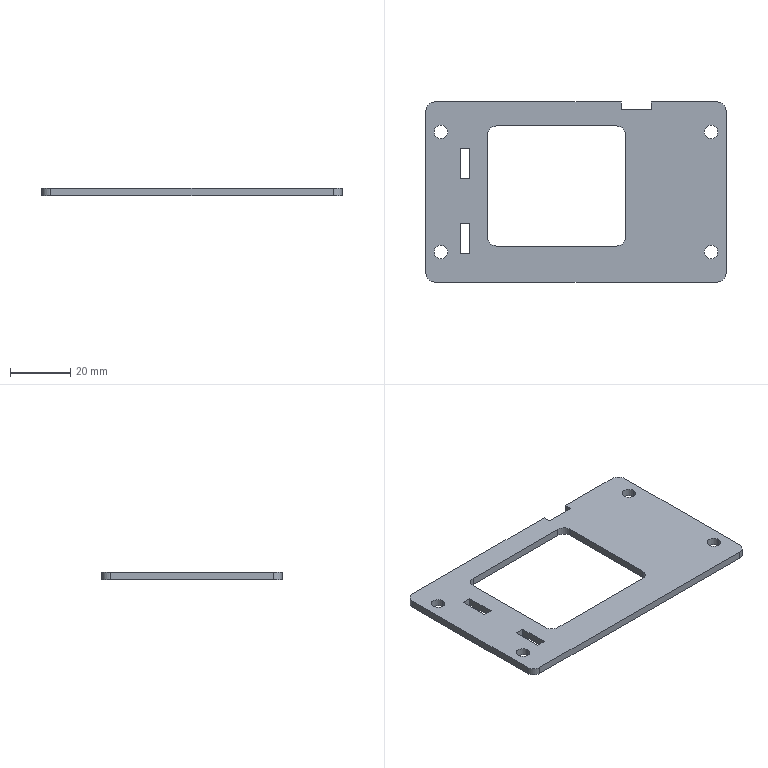Part | SolidWorks | features Cut 2, Fillet 2, ICE 2, MirrorPattern 2, FlatPattern 1, LPattern 1, SMBaseFlange 1, SheetMetal 1 | 1 solid | 38 faces | box 100 x 60 x 2.5 mm | volume 10028 mm3 | plane 22 | cylinder 16 | commonest cylinder face diameters 4.5 x8 6 x8
STEP:
#1=CARTESIAN_POINT('',(-42.75,20.,0.));
#2=VERTEX_POINT('',#1);
#3=CARTESIAN_POINT('',(-47.25,20.,0.));
#4=VERTEX_POINT('',#3);
#5=CARTESIAN_POINT('',(-45.,20.,0.));
#6=DIRECTION('',(0.,0.,-1.));
#7=DIRECTION('',(1.,0.,0.));
#8=AXIS2_PLACEMENT_3D('',#5,#6,#7);
#9=CIRCLE('',#8,2.25);
#10=EDGE_CURVE('',#2,#4,#9,.T.);
#11=ORIENTED_EDGE('',*,*,#10,.F.);
#12=CARTESIAN_POINT('',(-42.75,20.,-2.5));
#13=VERTEX_POINT('',#12);
#14=CARTESIAN_POINT('',(-42.75,20.,7.5));
#15=DIRECTION('',(0.,0.,-1.));
#16=VECTOR('',#15,1000.);
#17=LINE('',#14,#16);
#18=EDGE_CURVE('',#2,#13,#17,.T.);
#19=ORIENTED_EDGE('',*,*,#18,.T.);
#20=CARTESIAN_POINT('',(-47.25,20.,-2.5));
#21=VERTEX_POINT('',#20);
#22=CARTESIAN_POINT('',(-45.,20.,-2.5));
#23=DIRECTION('',(0.,0.,1.));
#24=DIRECTION('',(1.,0.,0.));
#25=AXIS2_PLACEMENT_3D('',#22,#23,#24);
#26=CIRCLE('',#25,2.25);
#27=EDGE_CURVE('',#21,#13,#26,.T.);
#28=ORIENTED_EDGE('',*,*,#27,.F.);
#29=CARTESIAN_POINT('',(-47.25,20.,7.5));
#30=DIRECTION('',(0.,0.,-1.));
#31=VECTOR('',#30,1000.);
#32=LINE('',#29,#31);
#33=EDGE_CURVE('',#4,#21,#32,.T.);
#34=ORIENTED_EDGE('',*,*,#33,.F.);
#35=EDGE_LOOP('',(#11,#19,#28,#34));
#36=FACE_OUTER_BOUND('',#35,.T.);
#37=CARTESIAN_POINT('',(-45.,20.,7.5));
#38=DIRECTION('',(0.,0.,-1.));
#39=DIRECTION('',(-1.,0.,0.));
#40=AXIS2_PLACEMENT_3D('',#37,#38,#39);
#41=CYLINDRICAL_SURFACE('',#40,2.25);
#42=ADVANCED_FACE('',(#36),#41,.F.);
#43=CARTESIAN_POINT('',(-47.25,-20.,0.));
#44=VERTEX_POINT('',#43);
#45=CARTESIAN_POINT('',(-42.75,-20.,0.));
#46=VERTEX_POINT('',#45);
#47=CARTESIAN_POINT('',(-45.,-20.,0.));
#48=DIRECTION('',(0.,0.,1.));
#49=DIRECTION('',(1.,0.,0.));
#50=AXIS2_PLACEMENT_3D('',#47,#48,#49);
#51=CIRCLE('',#50,2.25);
#52=EDGE_CURVE('',#44,#46,#51,.T.);
#53=ORIENTED_EDGE('',*,*,#52,.T.);
#54=CARTESIAN_POINT('',(-42.75,-20.,-2.5));
#55=VERTEX_POINT('',#54);
#56=CARTESIAN_POINT('',(-42.75,-20.,7.5));
#57=DIRECTION('',(0.,0.,-1.));
#58=VECTOR('',#57,1000.);
#59=LINE('',#56,#58);
#60=EDGE_CURVE('',#46,#55,#59,.T.);
#61=ORIENTED_EDGE('',*,*,#60,.T.);
#62=CARTESIAN_POINT('',(-47.25,-20.,-2.5));
#63=VERTEX_POINT('',#62);
#64=CARTESIAN_POINT('',(-45.,-20.,-2.5));
#65=DIRECTION('',(0.,0.,-1.));
#66=DIRECTION('',(1.,0.,0.));
#67=AXIS2_PLACEMENT_3D('',#64,#65,#66);
#68=CIRCLE('',#67,2.25);
#69=EDGE_CURVE('',#55,#63,#68,.T.);
#70=ORIENTED_EDGE('',*,*,#69,.T.);
#71=CARTESIAN_POINT('',(-47.25,-20.,7.5));
#72=DIRECTION('',(0.,0.,-1.));
#73=VECTOR('',#72,1000.);
#74=LINE('',#71,#73);
#75=EDGE_CURVE('',#44,#63,#74,.T.);
#76=ORIENTED_EDGE('',*,*,#75,.F.);
#77=EDGE_LOOP('',(#53,#61,#70,#76));
#78=FACE_OUTER_BOUND('',#77,.T.);
#79=CARTESIAN_POINT('',(-45.,-20.,7.5));
#80=DIRECTION('',(0.,0.,-1.));
#81=DIRECTION('',(-1.,0.,0.));
#82=AXIS2_PLACEMENT_3D('',#79,#80,#81);
#83=CYLINDRICAL_SURFACE('',#82,2.25);
#84=ADVANCED_FACE('',(#78),#83,.F.);
#85=CARTESIAN_POINT('',(47.25,-20.,0.));
#86=VERTEX_POINT('',#85);
#87=CARTESIAN_POINT('',(42.75,-20.,0.));
#88=VERTEX_POINT('',#87);
#89=CARTESIAN_POINT('',(45.,-20.,0.));
#90=DIRECTION('',(0.,0.,-1.));
#91=DIRECTION('',(1.,0.,0.));
#92=AXIS2_PLACEMENT_3D('',#89,#90,#91);
#93=CIRCLE('',#92,2.25);
#94=EDGE_CURVE('',#86,#88,#93,.T.);
#95=ORIENTED_EDGE('',*,*,#94,.F.);
#96=CARTESIAN_POINT('',(47.25,-20.,-2.5));
#97=VERTEX_POINT('',#96);
#98=CARTESIAN_POINT('',(47.25,-20.,7.5));
#99=DIRECTION('',(0.,0.,-1.));
#100=VECTOR('',#99,1000.);
#101=LINE('',#98,#100);
#102=EDGE_CURVE('',#86,#97,#101,.T.);
#103=ORIENTED_EDGE('',*,*,#102,.T.);
#104=CARTESIAN_POINT('',(42.75,-20.,-2.5));
#105=VERTEX_POINT('',#104);
#106=CARTESIAN_POINT('',(45.,-20.,-2.5));
#107=DIRECTION('',(0.,0.,1.));
#108=DIRECTION('',(-1.,0.,0.));
#109=AXIS2_PLACEMENT_3D('',#106,#107,#108);
#110=CIRCLE('',#109,2.25);
#111=EDGE_CURVE('',#105,#97,#110,.T.);
#112=ORIENTED_EDGE('',*,*,#111,.F.);
#113=CARTESIAN_POINT('',(42.75,-20.,7.5));
#114=DIRECTION('',(0.,0.,-1.));
#115=VECTOR('',#114,1000.);
#116=LINE('',#113,#115);
#117=EDGE_CURVE('',#88,#105,#116,.T.);
#118=ORIENTED_EDGE('',*,*,#117,.F.);
#119=EDGE_LOOP('',(#95,#103,#112,#118));
#120=FACE_OUTER_BOUND('',#119,.T.);
#121=CARTESIAN_POINT('',(45.,-20.,7.5));
#122=DIRECTION('',(0.,0.,-1.));
#123=DIRECTION('',(-1.,0.,0.));
#124=AXIS2_PLACEMENT_3D('',#121,#122,#123);
#125=CYLINDRICAL_SURFACE('',#124,2.25);
#126=ADVANCED_FACE('',(#120),#125,.F.);
#127=CARTESIAN_POINT('',(42.75,20.,0.));
#128=VERTEX_POINT('',#127);
#129=CARTESIAN_POINT('',(47.25,20.,0.));
#130=VERTEX_POINT('',#129);
#131=CARTESIAN_POINT('',(45.,20.,0.));
#132=DIRECTION('',(0.,0.,1.));
#133=DIRECTION('',(1.,0.,0.));
#134=AXIS2_PLACEMENT_3D('',#131,#132,#133);
#135=CIRCLE('',#134,2.25);
#136=EDGE_CURVE('',#128,#130,#135,.T.);
#137=ORIENTED_EDGE('',*,*,#136,.T.);
#138=CARTESIAN_POINT('',(47.25,20.,-2.5));
#139=VERTEX_POINT('',#138);
#140=CARTESIAN_POINT('',(47.25,20.,7.5));
#141=DIRECTION('',(0.,0.,-1.));
#142=VECTOR('',#141,1000.);
#143=LINE('',#140,#142);
#144=EDGE_CURVE('',#130,#139,#143,.T.);
#145=ORIENTED_EDGE('',*,*,#144,.T.);
#146=CARTESIAN_POINT('',(42.75,20.,-2.5));
#147=VERTEX_POINT('',#146);
#148=CARTESIAN_POINT('',(45.,20.,-2.5));
#149=DIRECTION('',(0.,0.,-1.));
#150=DIRECTION('',(-1.,0.,0.));
#151=AXIS2_PLACEMENT_3D('',#148,#149,#150);
#152=CIRCLE('',#151,2.25);
#153=EDGE_CURVE('',#139,#147,#152,.T.);
#154=ORIENTED_EDGE('',*,*,#153,.T.);
#155=CARTESIAN_POINT('',(42.75,20.,7.5));
#156=DIRECTION('',(0.,0.,-1.));
#157=VECTOR('',#156,1000.);
#158=LINE('',#155,#157);
#159=EDGE_CURVE('',#128,#147,#158,.T.);
#160=ORIENTED_EDGE('',*,*,#159,.F.);
#161=EDGE_LOOP('',(#137,#145,#154,#160));
#162=FACE_OUTER_BOUND('',#161,.T.);
#163=CARTESIAN_POINT('',(45.,20.,7.5));
#164=DIRECTION('',(0.,0.,-1.));
#165=DIRECTION('',(-1.,0.,0.));
#166=AXIS2_PLACEMENT_3D('',#163,#164,#165);
#167=CYLINDRICAL_SURFACE('',#166,2.25);
#168=ADVANCED_FACE('',(#162),#167,.F.);
#169=CARTESIAN_POINT('',(15.,30.,-2.5));
#170=VERTEX_POINT('',#169);
#171=CARTESIAN_POINT('',(15.,30.,0.));
#172=VERTEX_POINT('',#171);
#173=CARTESIAN_POINT('',(15.,30.,-2.5));
#174=DIRECTION('',(0.,0.,1.));
#175=VECTOR('',#174,1000.);
#176=LINE('',#173,#175);
#177=EDGE_CURVE('',#170,#172,#176,.T.);
#178=ORIENTED_EDGE('',*,*,#177,.F.);
#179=CARTESIAN_POINT('',(-47.,30.,-2.5));
#180=VERTEX_POINT('',#179);
#181=CARTESIAN_POINT('',(-50.,30.,-2.5));
#182=DIRECTION('',(-1.,0.,0.));
#183=VECTOR('',#182,1000.);
#184=LINE('',#181,#183);
#185=EDGE_CURVE('',#170,#180,#184,.T.);
#186=ORIENTED_EDGE('',*,*,#185,.T.);
#187=CARTESIAN_POINT('',(-47.,30.,0.));
#188=VERTEX_POINT('',#187);
#189=CARTESIAN_POINT('',(-47.,30.,-2.5));
#190=DIRECTION('',(0.,0.,1.));
#191=VECTOR('',#190,1000.);
#192=LINE('',#189,#191);
#193=EDGE_CURVE('',#180,#188,#192,.T.);
#194=ORIENTED_EDGE('',*,*,#193,.T.);
#195=CARTESIAN_POINT('',(-50.,30.,0.));
#196=DIRECTION('',(-1.,0.,0.));
#197=VECTOR('',#196,1000.);
#198=LINE('',#195,#197);
#199=EDGE_CURVE('',#172,#188,#198,.T.);
#200=ORIENTED_EDGE('',*,*,#199,.F.);
#201=EDGE_LOOP('',(#178,#186,#194,#200));
#202=FACE_OUTER_BOUND('',#201,.T.);
#203=CARTESIAN_POINT('',(-50.,30.,-2.5));
#204=DIRECTION('',(0.,1.,0.));
#205=DIRECTION('',(0.,0.,1.));
#206=AXIS2_PLACEMENT_3D('',#203,#204,#205);
#207=PLANE('',#206);
#208=ADVANCED_FACE('',(#202),#207,.T.);
#209=CARTESIAN_POINT('',(50.,-27.,0.));
#210=VERTEX_POINT('',#209);
#211=CARTESIAN_POINT('',(50.,27.,0.));
#212=VERTEX_POINT('',#211);
#213=CARTESIAN_POINT('',(50.,30.,0.));
#214=DIRECTION('',(0.,1.,0.));
#215=VECTOR('',#214,1000.);
#216=LINE('',#213,#215);
#217=EDGE_CURVE('',#210,#212,#216,.T.);
#218=ORIENTED_EDGE('',*,*,#217,.F.);
#219=CARTESIAN_POINT('',(50.,-27.,-2.5));
#220=VERTEX_POINT('',#219);
#221=CARTESIAN_POINT('',(50.,-27.,-2.5));
#222=DIRECTION('',(0.,0.,-1.));
#223=VECTOR('',#222,1000.);
#224=LINE('',#221,#223);
#225=EDGE_CURVE('',#210,#220,#224,.T.);
#226=ORIENTED_EDGE('',*,*,#225,.T.);
#227=CARTESIAN_POINT('',(50.,27.,-2.5));
#228=VERTEX_POINT('',#227);
#229=CARTESIAN_POINT('',(50.,30.,-2.5));
#230=DIRECTION('',(0.,1.,0.));
#231=VECTOR('',#230,1000.);
#232=LINE('',#229,#231);
#233=EDGE_CURVE('',#220,#228,#232,.T.);
#234=ORIENTED_EDGE('',*,*,#233,.T.);
#235=CARTESIAN_POINT('',(50.,27.,-2.5));
#236=DIRECTION('',(0.,0.,1.));
#237=VECTOR('',#236,1000.);
#238=LINE('',#235,#237);
#239=EDGE_CURVE('',#228,#212,#238,.T.);
#240=ORIENTED_EDGE('',*,*,#239,.T.);
#241=EDGE_LOOP('',(#218,#226,#234,#240));
#242=FACE_OUTER_BOUND('',#241,.T.);
#243=CARTESIAN_POINT('',(50.,30.,-2.5));
#244=DIRECTION('',(1.,0.,0.));
#245=DIRECTION('',(0.,1.,0.));
#246=AXIS2_PLACEMENT_3D('',#243,#244,#245);
#247=PLANE('',#246);
#248=ADVANCED_FACE('',(#242),#247,.T.);
#249=CARTESIAN_POINT('',(-47.,-30.,0.));
#250=VERTEX_POINT('',#249);
#251=CARTESIAN_POINT('',(47.,-30.,0.));
#252=VERTEX_POINT('',#251);
#253=CARTESIAN_POINT('',(-50.,-30.,0.));
#254=DIRECTION('',(1.,0.,0.));
#255=VECTOR('',#254,1000.);
#256=LINE('',#253,#255);
#257=EDGE_CURVE('',#250,#252,#256,.T.);
#258=ORIENTED_EDGE('',*,*,#257,.F.);
#259=CARTESIAN_POINT('',(-47.,-30.,-2.5));
#260=VERTEX_POINT('',#259);
#261=CARTESIAN_POINT('',(-47.,-30.,-2.5));
#262=DIRECTION('',(0.,0.,-1.));
#263=VECTOR('',#262,1000.);
#264=LINE('',#261,#263);
#265=EDGE_CURVE('',#250,#260,#264,.T.);
#266=ORIENTED_EDGE('',*,*,#265,.T.);
#267=CARTESIAN_POINT('',(47.,-30.,-2.5));
#268=VERTEX_POINT('',#267);
#269=CARTESIAN_POINT('',(-50.,-30.,-2.5));
#270=DIRECTION('',(1.,0.,0.));
#271=VECTOR('',#270,1000.);
#272=LINE('',#269,#271);
#273=EDGE_CURVE('',#260,#268,#272,.T.);
#274=ORIENTED_EDGE('',*,*,#273,.T.);
#275=CARTESIAN_POINT('',(47.,-30.,-2.5));
#276=DIRECTION('',(0.,0.,1.));
#277=VECTOR('',#276,1000.);
#278=LINE('',#275,#277);
#279=EDGE_CURVE('',#268,#252,#278,.T.);
#280=ORIENTED_EDGE('',*,*,#279,.T.);
#281=EDGE_LOOP('',(#258,#266,#274,#280));
#282=FACE_OUTER_BOUND('',#281,.T.);
#283=CARTESIAN_POINT('',(-50.,-30.,-2.5));
#284=DIRECTION('',(0.,-1.,0.));
#285=DIRECTION('',(0.,0.,-1.));
#286=AXIS2_PLACEMENT_3D('',#283,#284,#285);
#287=PLANE('',#286);
#288=ADVANCED_FACE('',(#282),#287,.T.);
#289=CARTESIAN_POINT('',(-50.,27.,-2.5));
#290=VERTEX_POINT('',#289);
#291=CARTESIAN_POINT('',(-50.,-27.,-2.5));
#292=VERTEX_POINT('',#291);
#293=CARTESIAN_POINT('',(-50.,30.,-2.5));
#294=DIRECTION('',(0.,-1.,0.));
#295=VECTOR('',#294,1000.);
#296=LINE('',#293,#295);
#297=EDGE_CURVE('',#290,#292,#296,.T.);
#298=ORIENTED_EDGE('',*,*,#297,.T.);
#299=CARTESIAN_POINT('',(-50.,-27.,0.));
#300=VERTEX_POINT('',#299);
#301=CARTESIAN_POINT('',(-50.,-27.,-2.5));
#302=DIRECTION('',(0.,0.,1.));
#303=VECTOR('',#302,1000.);
#304=LINE('',#301,#303);
#305=EDGE_CURVE('',#292,#300,#304,.T.);
#306=ORIENTED_EDGE('',*,*,#305,.T.);
#307=CARTESIAN_POINT('',(-50.,27.,0.));
#308=VERTEX_POINT('',#307);
#309=CARTESIAN_POINT('',(-50.,30.,0.));
#310=DIRECTION('',(0.,-1.,0.));
#311=VECTOR('',#310,1000.);
#312=LINE('',#309,#311);
#313=EDGE_CURVE('',#308,#300,#312,.T.);
#314=ORIENTED_EDGE('',*,*,#313,.F.);
#315=CARTESIAN_POINT('',(-50.,27.,-2.5));
#316=DIRECTION('',(0.,0.,-1.));
#317=VECTOR('',#316,1000.);
#318=LINE('',#315,#317);
#319=EDGE_CURVE('',#308,#290,#318,.T.);
#320=ORIENTED_EDGE('',*,*,#319,.T.);
#321=EDGE_LOOP('',(#298,#306,#314,#320));
#322=FACE_OUTER_BOUND('',#321,.T.);
#323=CARTESIAN_POINT('',(-50.,30.,-2.5));
#324=DIRECTION('',(-1.,0.,0.));
#325=DIRECTION('',(0.,-1.,0.));
#326=AXIS2_PLACEMENT_3D('',#323,#324,#325);
#327=PLANE('',#326);
#328=ADVANCED_FACE('',(#322),#327,.T.);
#329=CARTESIAN_POINT('',(25.,30.,0.));
#330=VERTEX_POINT('',#329);
#331=CARTESIAN_POINT('',(25.,30.,-2.5));
#332=VERTEX_POINT('',#331);
#333=CARTESIAN_POINT('',(25.,30.,-2.5));
#334=DIRECTION('',(0.,0.,-1.));
#335=VECTOR('',#334,1000.);
#336=LINE('',#333,#335);
#337=EDGE_CURVE('',#330,#332,#336,.T.);
#338=ORIENTED_EDGE('',*,*,#337,.F.);
#339=CARTESIAN_POINT('',(47.,30.,0.));
#340=VERTEX_POINT('',#339);
#341=CARTESIAN_POINT('',(-50.,30.,0.));
#342=DIRECTION('',(-1.,0.,0.));
#343=VECTOR('',#342,1000.);
#344=LINE('',#341,#343);
#345=EDGE_CURVE('',#340,#330,#344,.T.);
#346=ORIENTED_EDGE('',*,*,#345,.F.);
#347=CARTESIAN_POINT('',(47.,30.,-2.5));
#348=VERTEX_POINT('',#347);
#349=CARTESIAN_POINT('',(47.,30.,-2.5));
#350=DIRECTION('',(0.,0.,-1.));
#351=VECTOR('',#350,1000.);
#352=LINE('',#349,#351);
#353=EDGE_CURVE('',#340,#348,#352,.T.);
#354=ORIENTED_EDGE('',*,*,#353,.T.);
#355=CARTESIAN_POINT('',(-50.,30.,-2.5));
#356=DIRECTION('',(-1.,0.,0.));
#357=VECTOR('',#356,1000.);
#358=LINE('',#355,#357);
#359=EDGE_CURVE('',#348,#332,#358,.T.);
#360=ORIENTED_EDGE('',*,*,#359,.T.);
#361=EDGE_LOOP('',(#338,#346,#354,#360));
#362=FACE_OUTER_BOUND('',#361,.T.);
#363=CARTESIAN_POINT('',(-50.,30.,-2.5));
#364=DIRECTION('',(0.,1.,0.));
#365=DIRECTION('',(0.,0.,1.));
#366=AXIS2_PLACEMENT_3D('',#363,#364,#365);
#367=PLANE('',#366);
#368=ADVANCED_FACE('',(#362),#367,.T.);
#369=CARTESIAN_POINT('',(-26.5,22.,-2.5));
#370=VERTEX_POINT('',#369);
#371=CARTESIAN_POINT('',(13.5,22.,-2.5));
#372=VERTEX_POINT('',#371);
#373=CARTESIAN_POINT('',(-29.5,22.,-2.5));
#374=DIRECTION('',(1.,0.,0.));
#375=VECTOR('',#374,1000.);
#376=LINE('',#373,#375);
#377=EDGE_CURVE('',#370,#372,#376,.T.);
#378=ORIENTED_EDGE('',*,*,#377,.F.);
#379=CARTESIAN_POINT('',(-29.5,19.,-2.5));
#380=VERTEX_POINT('',#379);
#381=CARTESIAN_POINT('',(-26.5,19.,-2.5));
#382=DIRECTION('',(0.,0.,1.));
#383=DIRECTION('',(1.,0.,0.));
#384=AXIS2_PLACEMENT_3D('',#381,#382,#383);
#385=CIRCLE('',#384,3.);
#386=EDGE_CURVE('',#370,#380,#385,.T.);
#387=ORIENTED_EDGE('',*,*,#386,.T.);
#388=CARTESIAN_POINT('',(-29.5,-15.,-2.5));
#389=VERTEX_POINT('',#388);
#390=CARTESIAN_POINT('',(-29.5,-18.,-2.5));
#391=DIRECTION('',(0.,1.,0.));
#392=VECTOR('',#391,1000.);
#393=LINE('',#390,#392);
#394=EDGE_CURVE('',#389,#380,#393,.T.);
#395=ORIENTED_EDGE('',*,*,#394,.F.);
#396=CARTESIAN_POINT('',(-26.5,-18.,-2.5));
#397=VERTEX_POINT('',#396);
#398=CARTESIAN_POINT('',(-26.5,-15.,-2.5));
#399=DIRECTION('',(0.,0.,1.));
#400=DIRECTION('',(1.,0.,0.));
#401=AXIS2_PLACEMENT_3D('',#398,#399,#400);
#402=CIRCLE('',#401,3.);
#403=EDGE_CURVE('',#389,#397,#402,.T.);
#404=ORIENTED_EDGE('',*,*,#403,.T.);
#405=CARTESIAN_POINT('',(13.5,-18.,-2.5));
#406=VERTEX_POINT('',#405);
#407=CARTESIAN_POINT('',(-29.5,-18.,-2.5));
#408=DIRECTION('',(-1.,0.,0.));
#409=VECTOR('',#408,1000.);
#410=LINE('',#407,#409);
#411=EDGE_CURVE('',#406,#397,#410,.T.);
#412=ORIENTED_EDGE('',*,*,#411,.F.);
#413=CARTESIAN_POINT('',(16.5,-15.,-2.5));
#414=VERTEX_POINT('',#413);
#415=CARTESIAN_POINT('',(13.5,-15.,-2.5));
#416=DIRECTION('',(0.,0.,1.));
#417=DIRECTION('',(1.,0.,0.));
#418=AXIS2_PLACEMENT_3D('',#415,#416,#417);
#419=CIRCLE('',#418,3.);
#420=EDGE_CURVE('',#406,#414,#419,.T.);
#421=ORIENTED_EDGE('',*,*,#420,.T.);
#422=CARTESIAN_POINT('',(16.5,19.,-2.5));
#423=VERTEX_POINT('',#422);
#424=CARTESIAN_POINT('',(16.5,-18.,-2.5));
#425=DIRECTION('',(0.,-1.,0.));
#426=VECTOR('',#425,1000.);
#427=LINE('',#424,#426);
#428=EDGE_CURVE('',#423,#414,#427,.T.);
#429=ORIENTED_EDGE('',*,*,#428,.F.);
#430=CARTESIAN_POINT('',(13.5,19.,-2.5));
#431=DIRECTION('',(0.,0.,1.));
#432=DIRECTION('',(1.,0.,0.));
#433=AXIS2_PLACEMENT_3D('',#430,#431,#432);
#434=CIRCLE('',#433,3.);
#435=EDGE_CURVE('',#423,#372,#434,.T.);
#436=ORIENTED_EDGE('',*,*,#435,.T.);
#437=EDGE_LOOP('',(#378,#387,#395,#404,#412,#421,#429,#436));
#438=FACE_BOUND('',#437,.T.);
#439=ORIENTED_EDGE('',*,*,#27,.T.);
#440=CARTESIAN_POINT('',(-45.,20.,-2.5));
#441=DIRECTION('',(0.,0.,1.));
#442=DIRECTION('',(1.,0.,0.));
#443=AXIS2_PLACEMENT_3D('',#440,#441,#442);
#444=CIRCLE('',#443,2.25);
#445=EDGE_CURVE('',#13,#21,#444,.T.);
#446=ORIENTED_EDGE('',*,*,#445,.T.);
#447=EDGE_LOOP('',(#439,#446));
#448=FACE_BOUND('',#447,.T.);
#449=CARTESIAN_POINT('',(-45.,-20.,-2.5));
#450=DIRECTION('',(0.,0.,-1.));
#451=DIRECTION('',(1.,0.,0.));
#452=AXIS2_PLACEMENT_3D('',#449,#450,#451);
#453=CIRCLE('',#452,2.25);
#454=EDGE_CURVE('',#63,#55,#453,.T.);
#455=ORIENTED_EDGE('',*,*,#454,.F.);
#456=ORIENTED_EDGE('',*,*,#69,.F.);
#457=EDGE_LOOP('',(#455,#456));
#458=FACE_BOUND('',#457,.T.);
#459=ORIENTED_EDGE('',*,*,#111,.T.);
#460=CARTESIAN_POINT('',(45.,-20.,-2.5));
#461=DIRECTION('',(0.,0.,1.));
#462=DIRECTION('',(-1.,0.,0.));
#463=AXIS2_PLACEMENT_3D('',#460,#461,#462);
#464=CIRCLE('',#463,2.25);
#465=EDGE_CURVE('',#97,#105,#464,.T.);
#466=ORIENTED_EDGE('',*,*,#465,.T.);
#467=EDGE_LOOP('',(#459,#466));
#468=FACE_BOUND('',#467,.T.);
#469=CARTESIAN_POINT('',(45.,20.,-2.5));
#470=DIRECTION('',(0.,0.,-1.));
#471=DIRECTION('',(-1.,0.,0.));
#472=AXIS2_PLACEMENT_3D('',#469,#470,#471);
#473=CIRCLE('',#472,2.25);
#474=EDGE_CURVE('',#147,#139,#473,.T.);
#475=ORIENTED_EDGE('',*,*,#474,.F.);
#476=ORIENTED_EDGE('',*,*,#153,.F.);
#477=EDGE_LOOP('',(#475,#476));
#478=FACE_BOUND('',#477,.T.);
#479=CARTESIAN_POINT('',(-35.5,-20.5,-2.5));
#480=VERTEX_POINT('',#479);
#481=CARTESIAN_POINT('',(-38.5,-20.5,-2.5));
#482=VERTEX_POINT('',#481);
#483=CARTESIAN_POINT('',(-35.5,-20.5,-2.5));
#484=DIRECTION('',(-1.,0.,0.));
#485=VECTOR('',#484,1000.);
#486=LINE('',#483,#485);
#487=EDGE_CURVE('',#480,#482,#486,.T.);
#488=ORIENTED_EDGE('',*,*,#487,.F.);
#489=CARTESIAN_POINT('',(-35.5,-10.5,-2.5));
#490=VERTEX_POINT('',#489);
#491=CARTESIAN_POINT('',(-35.5,-20.5,-2.5));
#492=DIRECTION('',(0.,-1.,0.));
#493=VECTOR('',#492,1000.);
#494=LINE('',#491,#493);
#495=EDGE_CURVE('',#490,#480,#494,.T.);
#496=ORIENTED_EDGE('',*,*,#495,.F.);
#497=CARTESIAN_POINT('',(-38.5,-10.5,-2.5));
#498=VERTEX_POINT('',#497);
#499=CARTESIAN_POINT('',(-35.5,-10.5,-2.5));
#500=DIRECTION('',(1.,0.,0.));
#501=VECTOR('',#500,1000.);
#502=LINE('',#499,#501);
#503=EDGE_CURVE('',#498,#490,#502,.T.);
#504=ORIENTED_EDGE('',*,*,#503,.F.);
#505=CARTESIAN_POINT('',(-38.5,-20.5,-2.5));
#506=DIRECTION('',(0.,1.,0.));
#507=VECTOR('',#506,1000.);
#508=LINE('',#505,#507);
#509=EDGE_CURVE('',#482,#498,#508,.T.);
#510=ORIENTED_EDGE('',*,*,#509,.F.);
#511=EDGE_LOOP('',(#488,#496,#504,#510));
#512=FACE_BOUND('',#511,.T.);
#513=CARTESIAN_POINT('',(-35.5,4.5,-2.5));
#514=VERTEX_POINT('',#513);
#515=CARTESIAN_POINT('',(-38.5,4.5,-2.5));
#516=VERTEX_POINT('',#515);
#517=CARTESIAN_POINT('',(-35.5,4.5,-2.5));
#518=DIRECTION('',(-1.,0.,0.));
#519=VECTOR('',#518,1000.);
#520=LINE('',#517,#519);
#521=EDGE_CURVE('',#514,#516,#520,.T.);
#522=ORIENTED_EDGE('',*,*,#521,.F.);
#523=CARTESIAN_POINT('',(-35.5,14.5,-2.5));
#524=VERTEX_POINT('',#523);
#525=CARTESIAN_POINT('',(-35.5,4.5,-2.5));
#526=DIRECTION('',(0.,-1.,0.));
#527=VECTOR('',#526,1000.);
#528=LINE('',#525,#527);
#529=EDGE_CURVE('',#524,#514,#528,.T.);
#530=ORIENTED_EDGE('',*,*,#529,.F.);
#531=CARTESIAN_POINT('',(-38.5,14.5,-2.5));
#532=VERTEX_POINT('',#531);
#533=CARTESIAN_POINT('',(-35.5,14.5,-2.5));
#534=DIRECTION('',(1.,0.,0.));
#535=VECTOR('',#534,1000.);
#536=LINE('',#533,#535);
#537=EDGE_CURVE('',#532,#524,#536,.T.);
#538=ORIENTED_EDGE('',*,*,#537,.F.);
#539=CARTESIAN_POINT('',(-38.5,4.5,-2.5));
#540=DIRECTION('',(0.,1.,0.));
#541=VECTOR('',#540,1000.);
#542=LINE('',#539,#541);
#543=EDGE_CURVE('',#516,#532,#542,.T.);
#544=ORIENTED_EDGE('',*,*,#543,.F.);
#545=EDGE_LOOP('',(#522,#530,#538,#544));
#546=FACE_BOUND('',#545,.T.);
#547=ORIENTED_EDGE('',*,*,#185,.F.);
#548=CARTESIAN_POINT('',(15.,27.5,-2.5));
#549=VERTEX_POINT('',#548);
#550=CARTESIAN_POINT('',(15.,0.,-2.5));
#551=DIRECTION('',(0.,-1.,0.));
#552=VECTOR('',#551,1000.);
#553=LINE('',#550,#552);
#554=EDGE_CURVE('',#170,#549,#553,.T.);
#555=ORIENTED_EDGE('',*,*,#554,.T.);
#556=CARTESIAN_POINT('',(25.,27.5,-2.5));
#557=VERTEX_POINT('',#556);
#558=CARTESIAN_POINT('',(0.,27.5,-2.5));
#559=DIRECTION('',(1.,0.,0.));
#560=VECTOR('',#559,1000.);
#561=LINE('',#558,#560);
#562=EDGE_CURVE('',#549,#557,#561,.T.);
#563=ORIENTED_EDGE('',*,*,#562,.T.);
#564=CARTESIAN_POINT('',(25.,0.,-2.5));
#565=DIRECTION('',(0.,1.,0.));
#566=VECTOR('',#565,1000.);
#567=LINE('',#564,#566);
#568=EDGE_CURVE('',#557,#332,#567,.T.);
#569=ORIENTED_EDGE('',*,*,#568,.T.);
#570=ORIENTED_EDGE('',*,*,#359,.F.);
#571=CARTESIAN_POINT('',(47.,27.,-2.5));
#572=DIRECTION('',(0.,0.,-1.));
#573=DIRECTION('',(1.,0.,0.));
#574=AXIS2_PLACEMENT_3D('',#571,#572,#573);
#575=CIRCLE('',#574,3.);
#576=EDGE_CURVE('',#348,#228,#575,.T.);
#577=ORIENTED_EDGE('',*,*,#576,.T.);
#578=ORIENTED_EDGE('',*,*,#233,.F.);
#579=CARTESIAN_POINT('',(47.,-27.,-2.5));
#580=DIRECTION('',(0.,0.,-1.));
#581=DIRECTION('',(1.,0.,0.));
#582=AXIS2_PLACEMENT_3D('',#579,#580,#581);
#583=CIRCLE('',#582,3.);
#584=EDGE_CURVE('',#220,#268,#583,.T.);
#585=ORIENTED_EDGE('',*,*,#584,.T.);
#586=ORIENTED_EDGE('',*,*,#273,.F.);
#587=CARTESIAN_POINT('',(-47.,-27.,-2.5));
#588=DIRECTION('',(0.,0.,-1.));
#589=DIRECTION('',(1.,0.,0.));
#590=AXIS2_PLACEMENT_3D('',#587,#588,#589);
#591=CIRCLE('',#590,3.);
#592=EDGE_CURVE('',#260,#292,#591,.T.);
#593=ORIENTED_EDGE('',*,*,#592,.T.);
#594=ORIENTED_EDGE('',*,*,#297,.F.);
#595=CARTESIAN_POINT('',(-47.,27.,-2.5));
#596=DIRECTION('',(0.,0.,-1.));
#597=DIRECTION('',(1.,0.,0.));
#598=AXIS2_PLACEMENT_3D('',#595,#596,#597);
#599=CIRCLE('',#598,3.);
#600=EDGE_CURVE('',#290,#180,#599,.T.);
#601=ORIENTED_EDGE('',*,*,#600,.T.);
#602=EDGE_LOOP('',(#547,#555,#563,#569,#570,#577,#578,#585,#586,#593,#594,#601));
#603=FACE_OUTER_BOUND('',#602,.T.);
#604=CARTESIAN_POINT('',(0.,0.,-2.5));
#605=DIRECTION('',(0.,0.,1.));
#606=DIRECTION('',(1.,0.,0.));
#607=AXIS2_PLACEMENT_3D('',#604,#605,#606);
#608=PLANE('',#607);
#609=ADVANCED_FACE('',(#438,#448,#458,#468,#478,#512,#546,#603),#608,.F.);
#610=CARTESIAN_POINT('',(-29.5,19.,0.));
#611=VERTEX_POINT('',#610);
#612=CARTESIAN_POINT('',(-29.5,-15.,0.));
#613=VERTEX_POINT('',#612);
#614=CARTESIAN_POINT('',(-29.5,0.,0.));
#615=DIRECTION('',(0.,-1.,0.));
#616=VECTOR('',#615,1000.);
#617=LINE('',#614,#616);
#618=EDGE_CURVE('',#611,#613,#617,.T.);
#619=ORIENTED_EDGE('',*,*,#618,.F.);
#620=CARTESIAN_POINT('',(-26.5,22.,0.));
#621=VERTEX_POINT('',#620);
#622=CARTESIAN_POINT('',(-26.5,19.,0.));
#623=DIRECTION('',(0.,0.,-1.));
#624=DIRECTION('',(1.,0.,0.));
#625=AXIS2_PLACEMENT_3D('',#622,#623,#624);
#626=CIRCLE('',#625,3.);
#627=EDGE_CURVE('',#611,#621,#626,.T.);
#628=ORIENTED_EDGE('',*,*,#627,.T.);
#629=CARTESIAN_POINT('',(13.5,22.,0.));
#630=VERTEX_POINT('',#629);
#631=CARTESIAN_POINT('',(0.,22.,0.));
#632=DIRECTION('',(-1.,0.,0.));
#633=VECTOR('',#632,1000.);
#634=LINE('',#631,#633);
#635=EDGE_CURVE('',#630,#621,#634,.T.);
#636=ORIENTED_EDGE('',*,*,#635,.F.);
#637=CARTESIAN_POINT('',(16.5,19.,0.));
#638=VERTEX_POINT('',#637);
#639=CARTESIAN_POINT('',(13.5,19.,0.));
#640=DIRECTION('',(0.,0.,-1.));
#641=DIRECTION('',(1.,0.,0.));
#642=AXIS2_PLACEMENT_3D('',#639,#640,#641);
#643=CIRCLE('',#642,3.);
#644=EDGE_CURVE('',#630,#638,#643,.T.);
#645=ORIENTED_EDGE('',*,*,#644,.T.);
#646=CARTESIAN_POINT('',(16.5,-15.,0.));
#647=VERTEX_POINT('',#646);
#648=CARTESIAN_POINT('',(16.5,0.,0.));
#649=DIRECTION('',(0.,1.,0.));
#650=VECTOR('',#649,1000.);
#651=LINE('',#648,#650);
#652=EDGE_CURVE('',#647,#638,#651,.T.);
#653=ORIENTED_EDGE('',*,*,#652,.F.);
#654=CARTESIAN_POINT('',(13.5,-18.,0.));
#655=VERTEX_POINT('',#654);
#656=CARTESIAN_POINT('',(13.5,-15.,0.));
#657=DIRECTION('',(0.,0.,-1.));
#658=DIRECTION('',(1.,0.,0.));
#659=AXIS2_PLACEMENT_3D('',#656,#657,#658);
#660=CIRCLE('',#659,3.);
#661=EDGE_CURVE('',#647,#655,#660,.T.);
#662=ORIENTED_EDGE('',*,*,#661,.T.);
#663=CARTESIAN_POINT('',(-26.5,-18.,0.));
#664=VERTEX_POINT('',#663);
#665=CARTESIAN_POINT('',(0.,-18.,0.));
#666=DIRECTION('',(1.,0.,0.));
#667=VECTOR('',#666,1000.);
#668=LINE('',#665,#667);
#669=EDGE_CURVE('',#664,#655,#668,.T.);
#670=ORIENTED_EDGE('',*,*,#669,.F.);
#671=CARTESIAN_POINT('',(-26.5,-15.,0.));
#672=DIRECTION('',(0.,0.,-1.));
#673=DIRECTION('',(1.,0.,0.));
#674=AXIS2_PLACEMENT_3D('',#671,#672,#673);
#675=CIRCLE('',#674,3.);
#676=EDGE_CURVE('',#664,#613,#675,.T.);
#677=ORIENTED_EDGE('',*,*,#676,.T.);
#678=EDGE_LOOP('',(#619,#628,#636,#645,#653,#662,#670,#677));
#679=FACE_BOUND('',#678,.T.);
#680=CARTESIAN_POINT('',(-45.,20.,0.));
#681=DIRECTION('',(0.,0.,-1.));
#682=DIRECTION('',(1.,0.,0.));
#683=AXIS2_PLACEMENT_3D('',#680,#681,#682);
#684=CIRCLE('',#683,2.25);
#685=EDGE_CURVE('',#4,#2,#684,.T.);
#686=ORIENTED_EDGE('',*,*,#685,.T.);
#687=ORIENTED_EDGE('',*,*,#10,.T.);
#688=EDGE_LOOP('',(#686,#687));
#689=FACE_BOUND('',#688,.T.);
#690=ORIENTED_EDGE('',*,*,#52,.F.);
#691=CARTESIAN_POINT('',(-45.,-20.,0.));
#692=DIRECTION('',(0.,0.,1.));
#693=DIRECTION('',(1.,0.,0.));
#694=AXIS2_PLACEMENT_3D('',#691,#692,#693);
#695=CIRCLE('',#694,2.25);
#696=EDGE_CURVE('',#46,#44,#695,.T.);
#697=ORIENTED_EDGE('',*,*,#696,.F.);
#698=EDGE_LOOP('',(#690,#697));
#699=FACE_BOUND('',#698,.T.);
#700=CARTESIAN_POINT('',(45.,-20.,0.));
#701=DIRECTION('',(0.,0.,-1.));
#702=DIRECTION('',(1.,0.,0.));
#703=AXIS2_PLACEMENT_3D('',#700,#701,#702);
#704=CIRCLE('',#703,2.25);
#705=EDGE_CURVE('',#88,#86,#704,.T.);
#706=ORIENTED_EDGE('',*,*,#705,.T.);
#707=ORIENTED_EDGE('',*,*,#94,.T.);
#708=EDGE_LOOP('',(#706,#707));
#709=FACE_BOUND('',#708,.T.);
#710=ORIENTED_EDGE('',*,*,#136,.F.);
#711=CARTESIAN_POINT('',(45.,20.,0.));
#712=DIRECTION('',(0.,0.,1.));
#713=DIRECTION('',(1.,0.,0.));
#714=AXIS2_PLACEMENT_3D('',#711,#712,#713);
#715=CIRCLE('',#714,2.25);
#716=EDGE_CURVE('',#130,#128,#715,.T.);
#717=ORIENTED_EDGE('',*,*,#716,.F.);
#718=EDGE_LOOP('',(#710,#717));
#719=FACE_BOUND('',#718,.T.);
#720=CARTESIAN_POINT('',(-35.5,-20.5,0.));
#721=VERTEX_POINT('',#720);
#722=CARTESIAN_POINT('',(-35.5,-10.5,0.));
#723=VERTEX_POINT('',#722);
#724=CARTESIAN_POINT('',(-35.5,0.,0.));
#725=DIRECTION('',(0.,1.,0.));
#726=VECTOR('',#725,1000.);
#727=LINE('',#724,#726);
#728=EDGE_CURVE('',#721,#723,#727,.T.);
#729=ORIENTED_EDGE('',*,*,#728,.F.);
#730=CARTESIAN_POINT('',(-38.5,-20.5,0.));
#731=VERTEX_POINT('',#730);
#732=CARTESIAN_POINT('',(0.,-20.5,0.));
#733=DIRECTION('',(1.,0.,0.));
#734=VECTOR('',#733,1000.);
#735=LINE('',#732,#734);
#736=EDGE_CURVE('',#731,#721,#735,.T.);
#737=ORIENTED_EDGE('',*,*,#736,.F.);
#738=CARTESIAN_POINT('',(-38.5,-10.5,0.));
#739=VERTEX_POINT('',#738);
#740=CARTESIAN_POINT('',(-38.5,0.,0.));
#741=DIRECTION('',(0.,-1.,0.));
#742=VECTOR('',#741,1000.);
#743=LINE('',#740,#742);
#744=EDGE_CURVE('',#739,#731,#743,.T.);
#745=ORIENTED_EDGE('',*,*,#744,.F.);
#746=CARTESIAN_POINT('',(0.,-10.5,0.));
#747=DIRECTION('',(-1.,0.,0.));
#748=VECTOR('',#747,1000.);
#749=LINE('',#746,#748);
#750=EDGE_CURVE('',#723,#739,#749,.T.);
#751=ORIENTED_EDGE('',*,*,#750,.F.);
#752=EDGE_LOOP('',(#729,#737,#745,#751));
#753=FACE_BOUND('',#752,.T.);
#754=CARTESIAN_POINT('',(-35.5,4.5,0.));
#755=VERTEX_POINT('',#754);
#756=CARTESIAN_POINT('',(-35.5,14.5,0.));
#757=VERTEX_POINT('',#756);
#758=CARTESIAN_POINT('',(-35.5,0.,0.));
#759=DIRECTION('',(0.,1.,0.));
#760=VECTOR('',#759,1000.);
#761=LINE('',#758,#760);
#762=EDGE_CURVE('',#755,#757,#761,.T.);
#763=ORIENTED_EDGE('',*,*,#762,.F.);
#764=CARTESIAN_POINT('',(-38.5,4.5,0.));
#765=VERTEX_POINT('',#764);
#766=CARTESIAN_POINT('',(0.,4.5,0.));
#767=DIRECTION('',(1.,0.,0.));
#768=VECTOR('',#767,1000.);
#769=LINE('',#766,#768);
#770=EDGE_CURVE('',#765,#755,#769,.T.);
#771=ORIENTED_EDGE('',*,*,#770,.F.);
#772=CARTESIAN_POINT('',(-38.5,14.5,0.));
#773=VERTEX_POINT('',#772);
#774=CARTESIAN_POINT('',(-38.5,0.,0.));
#775=DIRECTION('',(0.,-1.,0.));
#776=VECTOR('',#775,1000.);
#777=LINE('',#774,#776);
#778=EDGE_CURVE('',#773,#765,#777,.T.);
#779=ORIENTED_EDGE('',*,*,#778,.F.);
#780=CARTESIAN_POINT('',(0.,14.5,0.));
#781=DIRECTION('',(-1.,0.,0.));
#782=VECTOR('',#781,1000.);
#783=LINE('',#780,#782);
#784=EDGE_CURVE('',#757,#773,#783,.T.);
#785=ORIENTED_EDGE('',*,*,#784,.F.);
#786=EDGE_LOOP('',(#763,#771,#779,#785));
#787=FACE_BOUND('',#786,.T.);
#788=CARTESIAN_POINT('',(15.,27.5,0.));
#789=VERTEX_POINT('',#788);
#790=CARTESIAN_POINT('',(15.,0.,0.));
#791=DIRECTION('',(0.,-1.,0.));
#792=VECTOR('',#791,1000.);
#793=LINE('',#790,#792);
#794=EDGE_CURVE('',#172,#789,#793,.T.);
#795=ORIENTED_EDGE('',*,*,#794,.F.);
#796=ORIENTED_EDGE('',*,*,#199,.T.);
#797=CARTESIAN_POINT('',(-47.,27.,0.));
#798=DIRECTION('',(0.,0.,1.));
#799=DIRECTION('',(1.,0.,0.));
#800=AXIS2_PLACEMENT_3D('',#797,#798,#799);
#801=CIRCLE('',#800,3.);
#802=EDGE_CURVE('',#188,#308,#801,.T.);
#803=ORIENTED_EDGE('',*,*,#802,.T.);
#804=ORIENTED_EDGE('',*,*,#313,.T.);
#805=CARTESIAN_POINT('',(-47.,-27.,0.));
#806=DIRECTION('',(0.,0.,1.));
#807=DIRECTION('',(1.,0.,0.));
#808=AXIS2_PLACEMENT_3D('',#805,#806,#807);
#809=CIRCLE('',#808,3.);
#810=EDGE_CURVE('',#300,#250,#809,.T.);
#811=ORIENTED_EDGE('',*,*,#810,.T.);
#812=ORIENTED_EDGE('',*,*,#257,.T.);
#813=CARTESIAN_POINT('',(47.,-27.,0.));
#814=DIRECTION('',(0.,0.,1.));
#815=DIRECTION('',(1.,0.,0.));
#816=AXIS2_PLACEMENT_3D('',#813,#814,#815);
#817=CIRCLE('',#816,3.);
#818=EDGE_CURVE('',#252,#210,#817,.T.);
#819=ORIENTED_EDGE('',*,*,#818,.T.);
#820=ORIENTED_EDGE('',*,*,#217,.T.);
#821=CARTESIAN_POINT('',(47.,27.,0.));
#822=DIRECTION('',(0.,0.,1.));
#823=DIRECTION('',(1.,0.,0.));
#824=AXIS2_PLACEMENT_3D('',#821,#822,#823);
#825=CIRCLE('',#824,3.);
#826=EDGE_CURVE('',#212,#340,#825,.T.);
#827=ORIENTED_EDGE('',*,*,#826,.T.);
#828=ORIENTED_EDGE('',*,*,#345,.T.);
#829=CARTESIAN_POINT('',(25.,27.5,0.));
#830=VERTEX_POINT('',#829);
#831=CARTESIAN_POINT('',(25.,33.638,0.));
#832=DIRECTION('',(0.,1.,0.));
#833=VECTOR('',#832,1000.);
#834=LINE('',#831,#833);
#835=EDGE_CURVE('',#830,#330,#834,.T.);
#836=ORIENTED_EDGE('',*,*,#835,.F.);
#837=CARTESIAN_POINT('',(15.,27.5,0.));
#838=DIRECTION('',(1.,0.,0.));
#839=VECTOR('',#838,1000.);
#840=LINE('',#837,#839);
#841=EDGE_CURVE('',#789,#830,#840,.T.);
#842=ORIENTED_EDGE('',*,*,#841,.F.);
#843=EDGE_LOOP('',(#795,#796,#803,#804,#811,#812,#819,#820,#827,#828,#836,#842));
#844=FACE_OUTER_BOUND('',#843,.T.);
#845=CARTESIAN_POINT('',(0.,0.,0.));
#846=DIRECTION('',(0.,0.,1.));
#847=DIRECTION('',(1.,0.,0.));
#848=AXIS2_PLACEMENT_3D('',#845,#846,#847);
#849=PLANE('',#848);
#850=ADVANCED_FACE('',(#679,#689,#699,#709,#719,#753,#787,#844),#849,.T.);
#851=ORIENTED_EDGE('',*,*,#592,.F.);
#852=ORIENTED_EDGE('',*,*,#265,.F.);
#853=ORIENTED_EDGE('',*,*,#810,.F.);
#854=ORIENTED_EDGE('',*,*,#305,.F.);
#855=EDGE_LOOP('',(#851,#852,#853,#854));
#856=FACE_OUTER_BOUND('',#855,.T.);
#857=CARTESIAN_POINT('',(-47.,-27.,-2.5));
#858=DIRECTION('',(0.,0.,1.));
#859=DIRECTION('',(1.,0.,0.));
#860=AXIS2_PLACEMENT_3D('',#857,#858,#859);
#861=CYLINDRICAL_SURFACE('',#860,3.);
#862=ADVANCED_FACE('',(#856),#861,.T.);
#863=ORIENTED_EDGE('',*,*,#584,.F.);
#864=ORIENTED_EDGE('',*,*,#225,.F.);
#865=ORIENTED_EDGE('',*,*,#818,.F.);
#866=ORIENTED_EDGE('',*,*,#279,.F.);
#867=EDGE_LOOP('',(#863,#864,#865,#866));
#868=FACE_OUTER_BOUND('',#867,.T.);
#869=CARTESIAN_POINT('',(47.,-27.,-2.5));
#870=DIRECTION('',(0.,0.,1.));
#871=DIRECTION('',(1.,0.,0.));
#872=AXIS2_PLACEMENT_3D('',#869,#870,#871);
#873=CYLINDRICAL_SURFACE('',#872,3.);
#874=ADVANCED_FACE('',(#868),#873,.T.);
#875=ORIENTED_EDGE('',*,*,#576,.F.);
#876=ORIENTED_EDGE('',*,*,#353,.F.);
#877=ORIENTED_EDGE('',*,*,#826,.F.);
#878=ORIENTED_EDGE('',*,*,#239,.F.);
#879=EDGE_LOOP('',(#875,#876,#877,#878));
#880=FACE_OUTER_BOUND('',#879,.T.);
#881=CARTESIAN_POINT('',(47.,27.,-2.5));
#882=DIRECTION('',(0.,0.,1.));
#883=DIRECTION('',(1.,0.,0.));
#884=AXIS2_PLACEMENT_3D('',#881,#882,#883);
#885=CYLINDRICAL_SURFACE('',#884,3.);
#886=ADVANCED_FACE('',(#880),#885,.T.);
#887=ORIENTED_EDGE('',*,*,#600,.F.);
#888=ORIENTED_EDGE('',*,*,#319,.F.);
#889=ORIENTED_EDGE('',*,*,#802,.F.);
#890=ORIENTED_EDGE('',*,*,#193,.F.);
#891=EDGE_LOOP('',(#887,#888,#889,#890));
#892=FACE_OUTER_BOUND('',#891,.T.);
#893=CARTESIAN_POINT('',(-47.,27.,-2.5));
#894=DIRECTION('',(0.,0.,1.));
#895=DIRECTION('',(1.,0.,0.));
#896=AXIS2_PLACEMENT_3D('',#893,#894,#895);
#897=CYLINDRICAL_SURFACE('',#896,3.);
#898=ADVANCED_FACE('',(#892),#897,.T.);
#899=CARTESIAN_POINT('',(15.,27.5,-10.));
#900=DIRECTION('',(0.,0.,1.));
#901=VECTOR('',#900,1000.);
#902=LINE('',#899,#901);
#903=EDGE_CURVE('',#549,#789,#902,.T.);
#904=ORIENTED_EDGE('',*,*,#903,.T.);
#905=ORIENTED_EDGE('',*,*,#841,.T.);
#906=CARTESIAN_POINT('',(25.,27.5,-10.));
#907=DIRECTION('',(0.,0.,1.));
#908=VECTOR('',#907,1000.);
#909=LINE('',#906,#908);
#910=EDGE_CURVE('',#557,#830,#909,.T.);
#911=ORIENTED_EDGE('',*,*,#910,.F.);
#912=ORIENTED_EDGE('',*,*,#562,.F.);
#913=EDGE_LOOP('',(#904,#905,#911,#912));
#914=FACE_OUTER_BOUND('',#913,.T.);
#915=CARTESIAN_POINT('',(15.,27.5,-10.));
#916=DIRECTION('',(0.,-1.,0.));
#917=DIRECTION('',(0.,0.,-1.));
#918=AXIS2_PLACEMENT_3D('',#915,#916,#917);
#919=PLANE('',#918);
#920=ADVANCED_FACE('',(#914),#919,.F.);
#921=ORIENTED_EDGE('',*,*,#177,.T.);
#922=ORIENTED_EDGE('',*,*,#794,.T.);
#923=ORIENTED_EDGE('',*,*,#903,.F.);
#924=ORIENTED_EDGE('',*,*,#554,.F.);
#925=EDGE_LOOP('',(#921,#922,#923,#924));
#926=FACE_OUTER_BOUND('',#925,.T.);
#927=CARTESIAN_POINT('',(15.,33.638,-10.));
#928=DIRECTION('',(-1.,0.,0.));
#929=DIRECTION('',(0.,0.,1.));
#930=AXIS2_PLACEMENT_3D('',#927,#928,#929);
#931=PLANE('',#930);
#932=ADVANCED_FACE('',(#926),#931,.F.);
#933=ORIENTED_EDGE('',*,*,#337,.T.);
#934=ORIENTED_EDGE('',*,*,#568,.F.);
#935=ORIENTED_EDGE('',*,*,#910,.T.);
#936=ORIENTED_EDGE('',*,*,#835,.T.);
#937=EDGE_LOOP('',(#933,#934,#935,#936));
#938=FACE_OUTER_BOUND('',#937,.T.);
#939=CARTESIAN_POINT('',(25.,33.638,-10.));
#940=DIRECTION('',(1.,0.,0.));
#941=DIRECTION('',(0.,1.,0.));
#942=AXIS2_PLACEMENT_3D('',#939,#940,#941);
#943=PLANE('',#942);
#944=ADVANCED_FACE('',(#938),#943,.F.);
#945=ORIENTED_EDGE('',*,*,#762,.T.);
#946=CARTESIAN_POINT('',(-35.5,14.5,7.5));
#947=DIRECTION('',(0.,0.,-1.));
#948=VECTOR('',#947,1000.);
#949=LINE('',#946,#948);
#950=EDGE_CURVE('',#757,#524,#949,.T.);
#951=ORIENTED_EDGE('',*,*,#950,.T.);
#952=ORIENTED_EDGE('',*,*,#529,.T.);
#953=CARTESIAN_POINT('',(-35.5,4.5,7.5));
#954=DIRECTION('',(0.,0.,-1.));
#955=VECTOR('',#954,1000.);
#956=LINE('',#953,#955);
#957=EDGE_CURVE('',#755,#514,#956,.T.);
#958=ORIENTED_EDGE('',*,*,#957,.F.);
#959=EDGE_LOOP('',(#945,#951,#952,#958));
#960=FACE_OUTER_BOUND('',#959,.T.);
#961=CARTESIAN_POINT('',(-35.5,4.5,7.5));
#962=DIRECTION('',(1.,0.,0.));
#963=DIRECTION('',(0.,1.,0.));
#964=AXIS2_PLACEMENT_3D('',#961,#962,#963);
#965=PLANE('',#964);
#966=ADVANCED_FACE('',(#960),#965,.F.);
#967=ORIENTED_EDGE('',*,*,#784,.T.);
#968=CARTESIAN_POINT('',(-38.5,14.5,7.5));
#969=DIRECTION('',(0.,0.,-1.));
#970=VECTOR('',#969,1000.);
#971=LINE('',#968,#970);
#972=EDGE_CURVE('',#773,#532,#971,.T.);
#973=ORIENTED_EDGE('',*,*,#972,.T.);
#974=ORIENTED_EDGE('',*,*,#537,.T.);
#975=ORIENTED_EDGE('',*,*,#950,.F.);
#976=EDGE_LOOP('',(#967,#973,#974,#975));
#977=FACE_OUTER_BOUND('',#976,.T.);
#978=CARTESIAN_POINT('',(-35.5,14.5,7.5));
#979=DIRECTION('',(0.,1.,0.));
#980=DIRECTION('',(0.,0.,1.));
#981=AXIS2_PLACEMENT_3D('',#978,#979,#980);
#982=PLANE('',#981);
#983=ADVANCED_FACE('',(#977),#982,.F.);
#984=ORIENTED_EDGE('',*,*,#778,.T.);
#985=CARTESIAN_POINT('',(-38.5,4.5,7.5));
#986=DIRECTION('',(0.,0.,-1.));
#987=VECTOR('',#986,1000.);
#988=LINE('',#985,#987);
#989=EDGE_CURVE('',#765,#516,#988,.T.);
#990=ORIENTED_EDGE('',*,*,#989,.T.);
#991=ORIENTED_EDGE('',*,*,#543,.T.);
#992=ORIENTED_EDGE('',*,*,#972,.F.);
#993=EDGE_LOOP('',(#984,#990,#991,#992));
#994=FACE_OUTER_BOUND('',#993,.T.);
#995=CARTESIAN_POINT('',(-38.5,4.5,7.5));
#996=DIRECTION('',(-1.,0.,0.));
#997=DIRECTION('',(0.,0.,1.));
#998=AXIS2_PLACEMENT_3D('',#995,#996,#997);
#999=PLANE('',#998);
#1000=ADVANCED_FACE('',(#994),#999,.F.);
#1001=ORIENTED_EDGE('',*,*,#770,.T.);
#1002=ORIENTED_EDGE('',*,*,#957,.T.);
#1003=ORIENTED_EDGE('',*,*,#521,.T.);
#1004=ORIENTED_EDGE('',*,*,#989,.F.);
#1005=EDGE_LOOP('',(#1001,#1002,#1003,#1004));
#1006=FACE_OUTER_BOUND('',#1005,.T.);
#1007=CARTESIAN_POINT('',(-35.5,4.5,7.5));
#1008=DIRECTION('',(0.,-1.,0.));
#1009=DIRECTION('',(0.,0.,-1.));
#1010=AXIS2_PLACEMENT_3D('',#1007,#1008,#1009);
#1011=PLANE('',#1010);
#1012=ADVANCED_FACE('',(#1006),#1011,.F.);
#1013=ORIENTED_EDGE('',*,*,#728,.T.);
#1014=CARTESIAN_POINT('',(-35.5,-10.5,7.5));
#1015=DIRECTION('',(0.,0.,-1.));
#1016=VECTOR('',#1015,1000.);
#1017=LINE('',#1014,#1016);
#1018=EDGE_CURVE('',#723,#490,#1017,.T.);
#1019=ORIENTED_EDGE('',*,*,#1018,.T.);
#1020=ORIENTED_EDGE('',*,*,#495,.T.);
#1021=CARTESIAN_POINT('',(-35.5,-20.5,7.5));
#1022=DIRECTION('',(0.,0.,-1.));
#1023=VECTOR('',#1022,1000.);
#1024=LINE('',#1021,#1023);
#1025=EDGE_CURVE('',#721,#480,#1024,.T.);
#1026=ORIENTED_EDGE('',*,*,#1025,.F.);
#1027=EDGE_LOOP('',(#1013,#1019,#1020,#1026));
#1028=FACE_OUTER_BOUND('',#1027,.T.);
#1029=CARTESIAN_POINT('',(-35.5,-20.5,7.5));
#1030=DIRECTION('',(1.,0.,0.));
#1031=DIRECTION('',(0.,1.,0.));
#1032=AXIS2_PLACEMENT_3D('',#1029,#1030,#1031);
#1033=PLANE('',#1032);
#1034=ADVANCED_FACE('',(#1028),#1033,.F.);
#1035=ORIENTED_EDGE('',*,*,#750,.T.);
#1036=CARTESIAN_POINT('',(-38.5,-10.5,7.5));
#1037=DIRECTION('',(0.,0.,-1.));
#1038=VECTOR('',#1037,1000.);
#1039=LINE('',#1036,#1038);
#1040=EDGE_CURVE('',#739,#498,#1039,.T.);
#1041=ORIENTED_EDGE('',*,*,#1040,.T.);
#1042=ORIENTED_EDGE('',*,*,#503,.T.);
#1043=ORIENTED_EDGE('',*,*,#1018,.F.);
#1044=EDGE_LOOP('',(#1035,#1041,#1042,#1043));
#1045=FACE_OUTER_BOUND('',#1044,.T.);
#1046=CARTESIAN_POINT('',(-35.5,-10.5,7.5));
#1047=DIRECTION('',(0.,1.,0.));
#1048=DIRECTION('',(0.,0.,1.));
#1049=AXIS2_PLACEMENT_3D('',#1046,#1047,#1048);
#1050=PLANE('',#1049);
#1051=ADVANCED_FACE('',(#1045),#1050,.F.);
#1052=ORIENTED_EDGE('',*,*,#744,.T.);
#1053=CARTESIAN_POINT('',(-38.5,-20.5,7.5));
#1054=DIRECTION('',(0.,0.,-1.));
#1055=VECTOR('',#1054,1000.);
#1056=LINE('',#1053,#1055);
#1057=EDGE_CURVE('',#731,#482,#1056,.T.);
#1058=ORIENTED_EDGE('',*,*,#1057,.T.);
#1059=ORIENTED_EDGE('',*,*,#509,.T.);
#1060=ORIENTED_EDGE('',*,*,#1040,.F.);
#1061=EDGE_LOOP('',(#1052,#1058,#1059,#1060));
#1062=FACE_OUTER_BOUND('',#1061,.T.);
#1063=CARTESIAN_POINT('',(-38.5,-20.5,7.5));
#1064=DIRECTION('',(-1.,0.,0.));
#1065=DIRECTION('',(0.,0.,1.));
#1066=AXIS2_PLACEMENT_3D('',#1063,#1064,#1065);
#1067=PLANE('',#1066);
#1068=ADVANCED_FACE('',(#1062),#1067,.F.);
#1069=ORIENTED_EDGE('',*,*,#736,.T.);
#1070=ORIENTED_EDGE('',*,*,#1025,.T.);
#1071=ORIENTED_EDGE('',*,*,#487,.T.);
#1072=ORIENTED_EDGE('',*,*,#1057,.F.);
#1073=EDGE_LOOP('',(#1069,#1070,#1071,#1072));
#1074=FACE_OUTER_BOUND('',#1073,.T.);
#1075=CARTESIAN_POINT('',(-35.5,-20.5,7.5));
#1076=DIRECTION('',(0.,-1.,0.));
#1077=DIRECTION('',(0.,0.,-1.));
#1078=AXIS2_PLACEMENT_3D('',#1075,#1076,#1077);
#1079=PLANE('',#1078);
#1080=ADVANCED_FACE('',(#1074),#1079,.F.);
#1081=ORIENTED_EDGE('',*,*,#144,.F.);
#1082=ORIENTED_EDGE('',*,*,#716,.T.);
#1083=ORIENTED_EDGE('',*,*,#159,.T.);
#1084=ORIENTED_EDGE('',*,*,#474,.T.);
#1085=EDGE_LOOP('',(#1081,#1082,#1083,#1084));
#1086=FACE_OUTER_BOUND('',#1085,.T.);
#1087=CARTESIAN_POINT('',(45.,20.,7.5));
#1088=DIRECTION('',(0.,0.,-1.));
#1089=DIRECTION('',(-1.,0.,0.));
#1090=AXIS2_PLACEMENT_3D('',#1087,#1088,#1089);
#1091=CYLINDRICAL_SURFACE('',#1090,2.25);
#1092=ADVANCED_FACE('',(#1086),#1091,.F.);
#1093=ORIENTED_EDGE('',*,*,#102,.F.);
#1094=ORIENTED_EDGE('',*,*,#705,.F.);
#1095=ORIENTED_EDGE('',*,*,#117,.T.);
#1096=ORIENTED_EDGE('',*,*,#465,.F.);
#1097=EDGE_LOOP('',(#1093,#1094,#1095,#1096));
#1098=FACE_OUTER_BOUND('',#1097,.T.);
#1099=CARTESIAN_POINT('',(45.,-20.,7.5));
#1100=DIRECTION('',(0.,0.,-1.));
#1101=DIRECTION('',(-1.,0.,0.));
#1102=AXIS2_PLACEMENT_3D('',#1099,#1100,#1101);
#1103=CYLINDRICAL_SURFACE('',#1102,2.25);
#1104=ADVANCED_FACE('',(#1098),#1103,.F.);
#1105=ORIENTED_EDGE('',*,*,#60,.F.);
#1106=ORIENTED_EDGE('',*,*,#696,.T.);
#1107=ORIENTED_EDGE('',*,*,#75,.T.);
#1108=ORIENTED_EDGE('',*,*,#454,.T.);
#1109=EDGE_LOOP('',(#1105,#1106,#1107,#1108));
#1110=FACE_OUTER_BOUND('',#1109,.T.);
#1111=CARTESIAN_POINT('',(-45.,-20.,7.5));
#1112=DIRECTION('',(0.,0.,-1.));
#1113=DIRECTION('',(-1.,0.,0.));
#1114=AXIS2_PLACEMENT_3D('',#1111,#1112,#1113);
#1115=CYLINDRICAL_SURFACE('',#1114,2.25);
#1116=ADVANCED_FACE('',(#1110),#1115,.F.);
#1117=ORIENTED_EDGE('',*,*,#18,.F.);
#1118=ORIENTED_EDGE('',*,*,#685,.F.);
#1119=ORIENTED_EDGE('',*,*,#33,.T.);
#1120=ORIENTED_EDGE('',*,*,#445,.F.);
#1121=EDGE_LOOP('',(#1117,#1118,#1119,#1120));
#1122=FACE_OUTER_BOUND('',#1121,.T.);
#1123=CARTESIAN_POINT('',(-45.,20.,7.5));
#1124=DIRECTION('',(0.,0.,-1.));
#1125=DIRECTION('',(-1.,0.,0.));
#1126=AXIS2_PLACEMENT_3D('',#1123,#1124,#1125);
#1127=CYLINDRICAL_SURFACE('',#1126,2.25);
#1128=ADVANCED_FACE('',(#1122),#1127,.F.);
#1129=ORIENTED_EDGE('',*,*,#618,.T.);
#1130=CARTESIAN_POINT('',(-29.5,-15.,-2.5));
#1131=DIRECTION('',(0.,0.,-1.));
#1132=VECTOR('',#1131,1000.);
#1133=LINE('',#1130,#1132);
#1134=EDGE_CURVE('',#613,#389,#1133,.T.);
#1135=ORIENTED_EDGE('',*,*,#1134,.T.);
#1136=ORIENTED_EDGE('',*,*,#394,.T.);
#1137=CARTESIAN_POINT('',(-29.5,19.,0.));
#1138=DIRECTION('',(0.,0.,1.));
#1139=VECTOR('',#1138,1000.);
#1140=LINE('',#1137,#1139);
#1141=EDGE_CURVE('',#380,#611,#1140,.T.);
#1142=ORIENTED_EDGE('',*,*,#1141,.T.);
#1143=EDGE_LOOP('',(#1129,#1135,#1136,#1142));
#1144=FACE_OUTER_BOUND('',#1143,.T.);
#1145=CARTESIAN_POINT('',(-29.5,-18.,7.5));
#1146=DIRECTION('',(-1.,0.,0.));
#1147=DIRECTION('',(0.,0.,1.));
#1148=AXIS2_PLACEMENT_3D('',#1145,#1146,#1147);
#1149=PLANE('',#1148);
#1150=ADVANCED_FACE('',(#1144),#1149,.F.);
#1151=ORIENTED_EDGE('',*,*,#669,.T.);
#1152=CARTESIAN_POINT('',(13.5,-18.,-2.5));
#1153=DIRECTION('',(0.,0.,-1.));
#1154=VECTOR('',#1153,1000.);
#1155=LINE('',#1152,#1154);
#1156=EDGE_CURVE('',#655,#406,#1155,.T.);
#1157=ORIENTED_EDGE('',*,*,#1156,.T.);
#1158=ORIENTED_EDGE('',*,*,#411,.T.);
#1159=CARTESIAN_POINT('',(-26.5,-18.,0.));
#1160=DIRECTION('',(0.,0.,1.));
#1161=VECTOR('',#1160,1000.);
#1162=LINE('',#1159,#1161);
#1163=EDGE_CURVE('',#397,#664,#1162,.T.);
#1164=ORIENTED_EDGE('',*,*,#1163,.T.);
#1165=EDGE_LOOP('',(#1151,#1157,#1158,#1164));
#1166=FACE_OUTER_BOUND('',#1165,.T.);
#1167=CARTESIAN_POINT('',(-29.5,-18.,7.5));
#1168=DIRECTION('',(0.,-1.,0.));
#1169=DIRECTION('',(0.,0.,-1.));
#1170=AXIS2_PLACEMENT_3D('',#1167,#1168,#1169);
#1171=PLANE('',#1170);
#1172=ADVANCED_FACE('',(#1166),#1171,.F.);
#1173=ORIENTED_EDGE('',*,*,#428,.T.);
#1174=CARTESIAN_POINT('',(16.5,-15.,0.));
#1175=DIRECTION('',(0.,0.,1.));
#1176=VECTOR('',#1175,1000.);
#1177=LINE('',#1174,#1176);
#1178=EDGE_CURVE('',#414,#647,#1177,.T.);
#1179=ORIENTED_EDGE('',*,*,#1178,.T.);
#1180=ORIENTED_EDGE('',*,*,#652,.T.);
#1181=CARTESIAN_POINT('',(16.5,19.,-2.5));
#1182=DIRECTION('',(0.,0.,-1.));
#1183=VECTOR('',#1182,1000.);
#1184=LINE('',#1181,#1183);
#1185=EDGE_CURVE('',#638,#423,#1184,.T.);
#1186=ORIENTED_EDGE('',*,*,#1185,.T.);
#1187=EDGE_LOOP('',(#1173,#1179,#1180,#1186));
#1188=FACE_OUTER_BOUND('',#1187,.T.);
#1189=CARTESIAN_POINT('',(16.5,-18.,7.5));
#1190=DIRECTION('',(1.,0.,0.));
#1191=DIRECTION('',(0.,0.,-1.));
#1192=AXIS2_PLACEMENT_3D('',#1189,#1190,#1191);
#1193=PLANE('',#1192);
#1194=ADVANCED_FACE('',(#1188),#1193,.F.);
#1195=ORIENTED_EDGE('',*,*,#635,.T.);
#1196=CARTESIAN_POINT('',(-26.5,22.,-2.5));
#1197=DIRECTION('',(0.,0.,-1.));
#1198=VECTOR('',#1197,1000.);
#1199=LINE('',#1196,#1198);
#1200=EDGE_CURVE('',#621,#370,#1199,.T.);
#1201=ORIENTED_EDGE('',*,*,#1200,.T.);
#1202=ORIENTED_EDGE('',*,*,#377,.T.);
#1203=CARTESIAN_POINT('',(13.5,22.,0.));
#1204=DIRECTION('',(0.,0.,1.));
#1205=VECTOR('',#1204,1000.);
#1206=LINE('',#1203,#1205);
#1207=EDGE_CURVE('',#372,#630,#1206,.T.);
#1208=ORIENTED_EDGE('',*,*,#1207,.T.);
#1209=EDGE_LOOP('',(#1195,#1201,#1202,#1208));
#1210=FACE_OUTER_BOUND('',#1209,.T.);
#1211=CARTESIAN_POINT('',(-29.5,22.,7.5));
#1212=DIRECTION('',(0.,1.,0.));
#1213=DIRECTION('',(0.,0.,1.));
#1214=AXIS2_PLACEMENT_3D('',#1211,#1212,#1213);
#1215=PLANE('',#1214);
#1216=ADVANCED_FACE('',(#1210),#1215,.F.);
#1217=ORIENTED_EDGE('',*,*,#661,.F.);
#1218=ORIENTED_EDGE('',*,*,#1178,.F.);
#1219=ORIENTED_EDGE('',*,*,#420,.F.);
#1220=ORIENTED_EDGE('',*,*,#1156,.F.);
#1221=EDGE_LOOP('',(#1217,#1218,#1219,#1220));
#1222=FACE_OUTER_BOUND('',#1221,.T.);
#1223=CARTESIAN_POINT('',(13.5,-15.,7.5));
#1224=DIRECTION('',(0.,0.,1.));
#1225=DIRECTION('',(1.,0.,0.));
#1226=AXIS2_PLACEMENT_3D('',#1223,#1224,#1225);
#1227=CYLINDRICAL_SURFACE('',#1226,3.);
#1228=ADVANCED_FACE('',(#1222),#1227,.F.);
#1229=ORIENTED_EDGE('',*,*,#676,.F.);
#1230=ORIENTED_EDGE('',*,*,#1163,.F.);
#1231=ORIENTED_EDGE('',*,*,#403,.F.);
#1232=ORIENTED_EDGE('',*,*,#1134,.F.);
#1233=EDGE_LOOP('',(#1229,#1230,#1231,#1232));
#1234=FACE_OUTER_BOUND('',#1233,.T.);
#1235=CARTESIAN_POINT('',(-26.5,-15.,7.5));
#1236=DIRECTION('',(0.,0.,1.));
#1237=DIRECTION('',(1.,0.,0.));
#1238=AXIS2_PLACEMENT_3D('',#1235,#1236,#1237);
#1239=CYLINDRICAL_SURFACE('',#1238,3.);
#1240=ADVANCED_FACE('',(#1234),#1239,.F.);
#1241=ORIENTED_EDGE('',*,*,#627,.F.);
#1242=ORIENTED_EDGE('',*,*,#1141,.F.);
#1243=ORIENTED_EDGE('',*,*,#386,.F.);
#1244=ORIENTED_EDGE('',*,*,#1200,.F.);
#1245=EDGE_LOOP('',(#1241,#1242,#1243,#1244));
#1246=FACE_OUTER_BOUND('',#1245,.T.);
#1247=CARTESIAN_POINT('',(-26.5,19.,7.5));
#1248=DIRECTION('',(0.,0.,1.));
#1249=DIRECTION('',(1.,0.,0.));
#1250=AXIS2_PLACEMENT_3D('',#1247,#1248,#1249);
#1251=CYLINDRICAL_SURFACE('',#1250,3.);
#1252=ADVANCED_FACE('',(#1246),#1251,.F.);
#1253=ORIENTED_EDGE('',*,*,#644,.F.);
#1254=ORIENTED_EDGE('',*,*,#1207,.F.);
#1255=ORIENTED_EDGE('',*,*,#435,.F.);
#1256=ORIENTED_EDGE('',*,*,#1185,.F.);
#1257=EDGE_LOOP('',(#1253,#1254,#1255,#1256));
#1258=FACE_OUTER_BOUND('',#1257,.T.);
#1259=CARTESIAN_POINT('',(13.5,19.,7.5));
#1260=DIRECTION('',(0.,0.,1.));
#1261=DIRECTION('',(1.,0.,0.));
#1262=AXIS2_PLACEMENT_3D('',#1259,#1260,#1261);
#1263=CYLINDRICAL_SURFACE('',#1262,3.);
#1264=ADVANCED_FACE('',(#1258),#1263,.F.);
#1265=CLOSED_SHELL('',(#42,#84,#126,#168,#208,#248,#288,#328,#368,#609,#850,#862,#874,#886,#898,#920,#932,#944,#966,#983,#1000,#1012,#1034,#1051,#1068,#1080,#1092,#1104,#1116,#1128,#1150,#1172,#1194,#1216,#1228,#1240,#1252,#1264));
#1266=MANIFOLD_SOLID_BREP('',#1265);
#1267=CARTESIAN_POINT('',(0.,0.,0.));
#1268=DIRECTION('',(0.,0.,1.));
#1269=DIRECTION('',(1.,0.,0.));
#1270=AXIS2_PLACEMENT_3D('',#1267,#1268,#1269);
#1271=(LENGTH_UNIT()NAMED_UNIT(*)SI_UNIT(.MILLI.,.METRE.));
#1272=UNCERTAINTY_MEASURE_WITH_UNIT(LENGTH_MEASURE(0.00001),#1271,'','');
#1273=(NAMED_UNIT(*)PLANE_ANGLE_UNIT()SI_UNIT($,.RADIAN.));
#1274=(NAMED_UNIT(*)SI_UNIT($,.STERADIAN.)SOLID_ANGLE_UNIT());
#1275=(GEOMETRIC_REPRESENTATION_CONTEXT(3)GLOBAL_UNCERTAINTY_ASSIGNED_CONTEXT((#1272))GLOBAL_UNIT_ASSIGNED_CONTEXT((#1271,#1273,#1274))REPRESENTATION_CONTEXT('',''));
#1276=ADVANCED_BREP_SHAPE_REPRESENTATION('',(#1266,#1270),#1275);